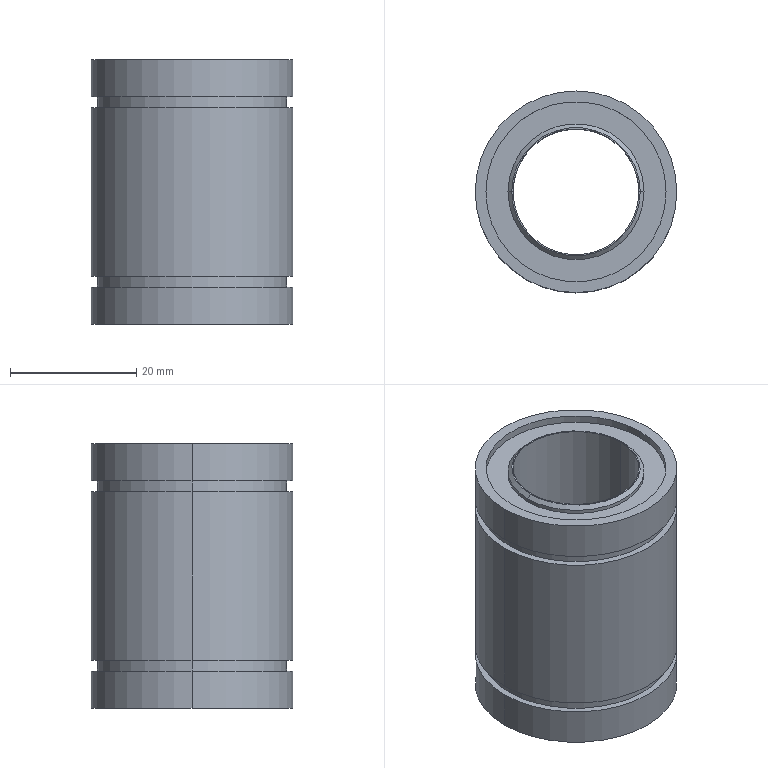Part | STEP file | bore 20 linear bearing | 1 solid | 34 faces | box 32 x 32 x 42 mm | volume 19566 mm3 | cylinder 20 | plane 10 | cone 4 | commonest cylinder face diameters 32 x6 21.6 x4 28.6 x4 30 x4 20 x2